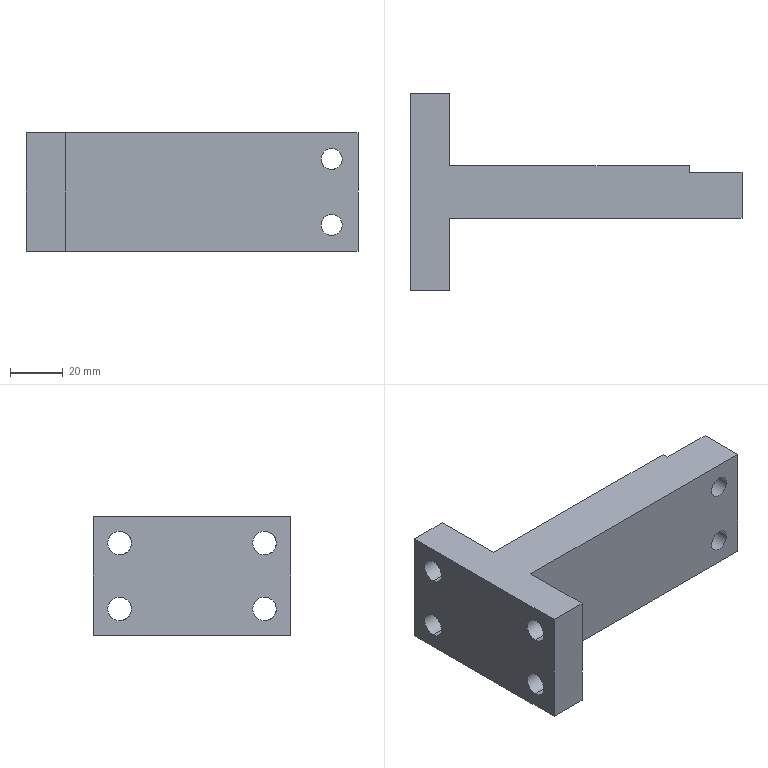Part | STEP file | Positioning_id2266_x_t | 1 solid | 24 faces | box 126.002 x 75 x 45 mm | volume 142700 mm3 | cylinder 12 | plane 12 | commonest cylinder face diameters 9 x8 8 x4